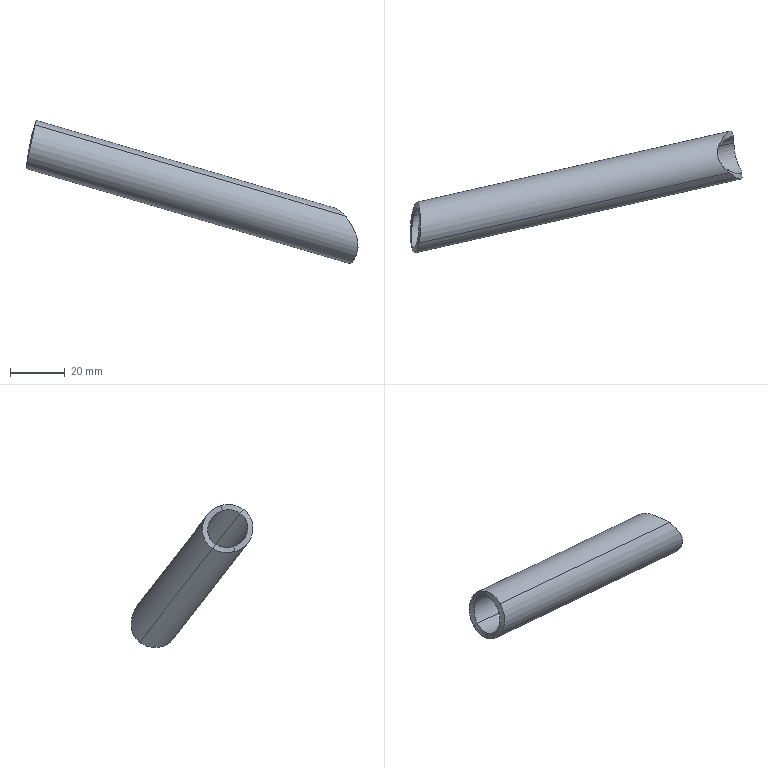Part | SolidWorks | features BaseBody 1 | 1 solid | 15 faces | box 121.583 x 44.725 x 52.421 mm | volume 12378 mm3 | spline 11 | cylinder 4 | commonest cylinder face diameters 14 x2 18 x2